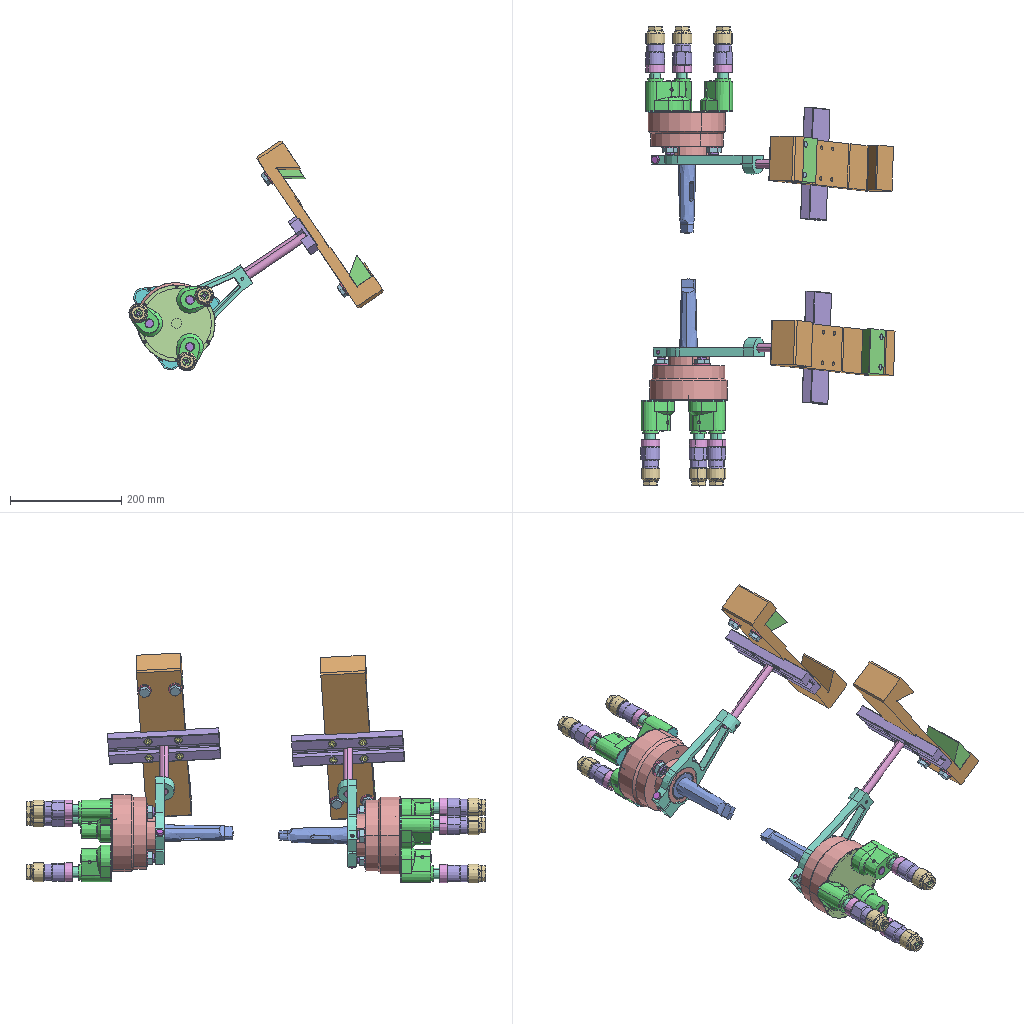Assembly | SolidWorks | 34 different items | 143 placed | box 457 x 827 x 414 mm
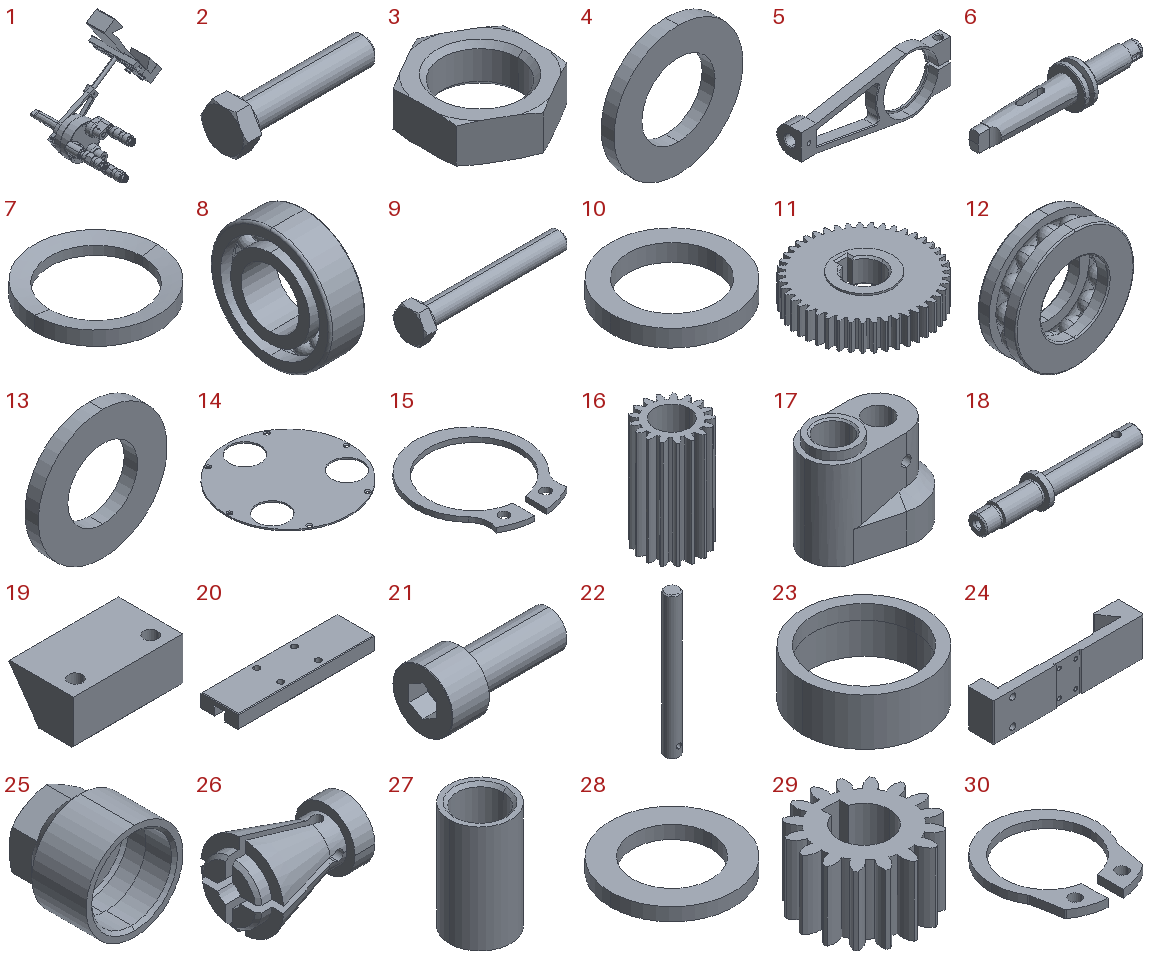Parts list (item | name | quantity | parent item | size | volume | features):
1 | (subassembly) | x2 | - | 456.998 x 372.31 x 409.469 mm | 2395331 mm3 | features ReferencePattern 32, CompositeCurve 27, LocalCirPattern 3
2 | - | x4 | in 1 | 62.5 x 20.785 x 18 mm | 8272 mm3 | features RevCut 4, Chamfer 1, Extrusion 1, Fillet 1, LPattern 1, Revolution 1
3 | - | x6 | in 1 | 23.219 x 26.75 x 8 mm | 2049 mm3 | features Cut 2, Chamfer 1, Extrusion 1
4 | - | x6 | in 1 | 30 x 3 x 30 mm | 1440 mm3 | features Revolution 1
5 | - | x2 | in 1 | 210 x 34 x 82 mm | 81908 mm3 | features ICE 6, Chamfer 3, Fillet 2, HoleWzd 2, CutThin 1, ExtruRefSurface 1, Extrusion 1
6 | - | x2 | in 1 | 216 x 51 x 51 mm | 132474 mm3 | features ICE 5, Chamfer 1, MirrorPattern 1, Revolution 1, SweepCut 1
7 | - | x2 | in 1 | 52 x 52 x 6 mm | 4561 mm3 | features Extrusion 1, ICE 1, MirrorPattern 1
8 | - | x4 | in 1 | 15 x 52 x 52 mm | 16133 mm3 | features Revolution 3, Fillet 2, CirPattern 1
9 | - | x2 | in 1 | 65.3 x 15.011 x 13 mm | 3770 mm3 | features RevCut 4, Chamfer 1, Extrusion 1, Fillet 1, LPattern 1, Revolution 1
10 | - | x2 | in 1 | 36 x 36 x 5 mm | 2536 mm3 | features Extrusion 1
11 | - | x2 | in 1 | 70.282 x 70.32 x 16 mm | 46691 mm3 | features ICE 4, Chamfer 1, CirPattern 1, Extrusion 1
12 | - | x6 | in 1 | 28 x 9 x 28 mm | 2845 mm3 | features Revolution 3, CirPattern 1, Fillet 1
13 | - | x4 | in 1 | 24 x 2.5 x 24 mm | 799.143 mm3 | features Revolution 1
14 | - | x2 | in 1 | 139 x 139 x 1.5 mm | 18307 mm3 | features ICE 3, CirPattern 2, Extrusion 1
15 | - | x6 | in 1 | 22.5 x 25.566 x 1 mm | 158.597 mm3 | features Extrusion 1
16 | - | x6 | in 1 | 28.328 x 28.443 x 49.5 mm | 14667 mm3 | features CirPattern 1, Extrusion 1, ICE 1
17 | - | x6 | in 1 | 68 x 48 x 58 mm | 60377 mm3 | features ICE 7, Chamfer 2, Extrusion 1, HoleWzd 1
18 | - | x6 | in 1 | 133 x 25 x 25 mm | 28520 mm3 | features ICE 3, Chamfer 2, RevCut 1, Revolution 1
19 | - | x2 | in 1 | 80 x 46.833 x 32 mm | 87358 mm3 | features Chamfer 1, Extrusion 1, HoleWzd 1, MirrorPattern 1
20 | - | x2 | in 1 | 200 x 55 x 20 mm | 170246 mm3 | features MirrorPattern 2, Chamfer 1, Extrusion 1, HoleWzd 1
21 | - | x8 | in 1 | 28 x 13 x 13 mm | 1937 mm3 | features BlendCut 1, Cut 1, Fillet 1, LPattern 1, RevCut 1, Revolution 1
22 | - | x2 | in 1 | 15 x 15 x 150 mm | 26172 mm3 | features Chamfer 1, ExtruRefSurface 1, Extrusion 1, HoleWzd 1
23 | - | x6 | in 1 | 34 x 34 x 13 mm | 3395 mm3 | features Extrusion 1, ICE 1
24 | - | x2 | in 1 | 320 x 55 x 80 mm | 674156 mm3 | features ICE 3, MirrorPattern 2, Chamfer 1, Extrusion 1, HoleWzd 1
25 | - | x6 | in 1 | 34 x 32 x 34 mm | 9791 mm3 | features ICE 6, Chamfer 2, Extrusion 1, HoleWzd 1
26 | - | x6 | in 1 | 35 x 24.92 x 24.92 mm | 6477 mm3 | features ICE 5, Chamfer 1, Revolution 1
27 | - | x6 | in 1 | 20 x 20 x 35 mm | 4761 mm3 | features Chamfer 1, Extrusion 1
28 | - | x6 | in 1 | 23.5 x 23.5 x 2.5 mm | 642.554 mm3 | features Extrusion 1
29 | - | x6 | in 1 | 26.937 x 26.937 x 16 mm | 5099 mm3 | features ICE 2, CirPattern 1, Extrusion 1
30 | - | x6 | in 1 | 13.6 x 15.973 x 1 mm | 68.14 mm3 | features Extrusion 1
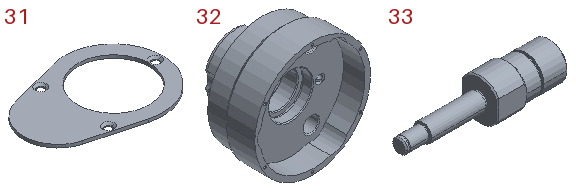31 | - | x6 | in 1 | 68 x 48 x 1.5 mm | 2249 mm3 | features ICE 5, Extrusion 1
32 | - | x2 | in 1 | 139 x 94 x 139 mm | 531526 mm3 | features Chamfer 3, ICE 3, CirPattern 2, RevCut 2, SweepCut 2, HoleWzd 1, Revolution 1
33 | - | x6 | in 1 | 124 x 30 x 34 mm | 43283 mm3 | features Chamfer 2, ICE 2, RevCut 1, Revolution 1
34 | Base Plate | x1 | - | - | - | -
Mates (type | each side: item.copy, entity, surface, feature):
Concentric | 6.1 edge | 7.1 edge
Coincident | 6.1 face cone Revolve1 | 7.1 edge
Concentric | 32.1 edge | 6.1 edge
Coincident | 32.1 face plane Revolve1 | 6.1 face plane Revolve1
Concentric | 32.1 edge | 5.1 edge
Coincident | 32.1 face plane Revolve1 | 5.1 face plane Cut-Extrude3
Concentric | 22.1 edge | 5.1 edge
Coincident | 22.1 face plane Boss-Extrude1 | 5.1 face plane Boss-Extrude2
Concentric | 22.1 face cylinder Ø5.0mm Blind Hole1 | 5.1 face cylinder Ø5.0mm Blind Hole1
Coincident | 22.1 face plane Boss-Extrude1 | 20.1 face plane Boss-Extrude1
Width | 20.1 face plane Boss-Extrude1 | 20.1 face plane Boss-Extrude1 | 22.1 face cylinder Boss-Extrude1 | 2 times
Coincident | 24.1 face plane Cut-Extrude2 | 20.1 face plane Boss-Extrude1
Concentric | 24.1 edge | 20.1 edge | 2 times
Coincident | 24.1 face plane Cut-Extrude1 | 19.1 face plane Boss-Extrude1
Concentric | 24.1 face cylinder Cut-Extrude3 | 19.1 edge | 2 times
Concentric | 24.1 face cylinder Cut-Extrude3 | 2.1 face cylinder Boss-Revolve1
Coincident | 19.1 face plane Boss-Extrude1 | 2.1 face plane Boss-Revolve1
Coincident | 24.1 face plane Boss-Extrude1 | 13.1 face plane Base-Revolve
Concentric | 13.1 face cylinder Base-Revolve | 2.1 face cylinder Boss-Revolve1
Concentric | 2.2 face cylinder Boss-Revolve1 | 13.2 face cylinder Base-Revolve
Coincident | 2.2 face plane Base-Extrude | 13.2 face plane Base-Revolve
Concentric | 24.1 face cylinder Cut-Extrude3 | 2.2 face cylinder Boss-Revolve1
Coincident | 19.1 face plane Boss-Extrude1 | 2.2 face plane Boss-Revolve1
Concentric | 24.1 face cylinder Mirror2 | 21.1 face cylinder Base-Revolve
Coincident | 20.1 face plane Mirror2 | 21.1 face plane Base-Revolve
Concentric | 20.1 face cylinder Mirror2 | 21.2 face cylinder Base-Revolve
Concentric | 20.1 face cylinder Hole5 | 21.3 face cylinder Base-Revolve
Concentric | 20.1 face cylinder Mirror1 | 21.4 face cylinder Base-Revolve
Coincident | 20.1 face plane Mirror1 | 21.4 face plane Base-Revolve
Coincident | 20.1 face plane Hole5 | 21.3 face plane Base-Revolve
Coincident | 20.1 face plane Mirror2 | 21.2 face plane Base-Revolve
Concentric | 5.1 face cylinder Cut-Extrude4 | 9.1 face cylinder Boss-Revolve1
Coincident | 5.1 face plane Boss-Extrude1 | 9.1 face plane Base-Extrude
Concentric | 6.1 face cylinder Revolve1 | 8.1 face cylinder Base-Revolve
Coincident | 32.1 face plane Cut-Revolve1 | 8.1 face plane Base-Revolve
Concentric | 32.1 face cylinder Cut-Revolve1 | 11.1 face cylinder Cut-Extrude2
Concentric | 6.1 face cylinder Revolve1 | 8.2 face cylinder Boss-Revolve2
Concentric | 6.1 face cylinder Revolve1 | 10.1 face cylinder Boss-Extrude1
Coincident | 32.1 face plane Cut-Revolve1 | 8.2 face plane Base-Revolve
Coincident | 8.2 face plane Boss-Revolve2 | 10.1 face plane Boss-Extrude1
Coincident | 11.1 face plane Cut-Extrude2 | 10.1 face plane Boss-Extrude1
Concentric | 32.1 face cylinder Revolve1 | 14.1 face cylinder Boss-Extrude1
Concentric | 32.1 edge | 14.1 edge
Concentric | 6.1 edge | 15.1 edge
Coincident | 6.1 face plane Revolve1 | 15.1 face plane Base-Extrude
Coincident | 32.1 face plane Revolve1 | 14.1 face plane Boss-Extrude1
Concentric | 31.1 edge | 17.1 edge | 2 times
Coincident | 31.1 face plane Boss-Extrude1 | 17.1 face plane Boss-Extrude1
Concentric | 14.1 face cylinder Cut-Extrude1 | 31.1 face cylinder Cut-Extrude1
Coincident | 14.1 face plane Boss-Extrude1 | 31.1 face plane Boss-Extrude1
Concentric | 18.1 face cylinder Revolve1 | 17.1 face cylinder Cut-Extrude3
Concentric | 18.1 face cylinder Cut-Extrude1 | 17.1 face cylinder Cut-Extrude5
Concentric | 17.1 edge | 29.1 edge
Concentric | 17.1 face cylinder Cut-Extrude1 | 30.1 edge
Concentric | 25.1 face cylinder M30x2.0 Tapped Hole1 | 17.1 face cylinder Cut-Extrude1
Concentric | 17.1 face cylinder Cut-Extrude1 | 28.1 face cylinder Boss-Extrude1
Concentric | 17.1 face cylinder Cut-Extrude1 | 27.1 face cylinder Boss-Extrude1
Concentric | 17.1 face cylinder Cut-Extrude1 | 23.1 face cylinder Cut-Extrude1
Concentric | 17.1 face cylinder Cut-Extrude1 | 33.1 face cylinder Revolve1
Coincident | 30.1 face plane Base-Extrude | 33.1 face plane Revolve1
Concentric | 12.1 face cylinder Boss-Revolve3 | 33.1 face cylinder Revolve1
Coincident | 12.1 face plane Base-Revolve | 33.1 face plane Revolve1
Coincident | 29.1 face plane Boss-Extrude1 | 33.1 face plane Revolve1
Coincident | 29.1 face plane Boss-Extrude1 | 28.1 face plane Boss-Extrude1
Coincident | 28.1 face plane Boss-Extrude1 | 27.1 face plane Boss-Extrude1
Coincident | 23.1 face plane Boss-Extrude1 | 33.1 face plane Revolve1
Concentric | 33.1 face cone Cut-Revolve1 | 26.1 face cylinder Revolve1
Coincident | 33.1 edge | 26.1 face plane Revolve1
Coincident | 25.1 face plane Boss-Extrude2 | 33.1 face plane Revolve1
Coincident | 4.1 face plane Base-Revolve | 3.1 face plane Base-Extrude
Concentric | 4.1 face cylinder Base-Revolve | 3.1 face cylinder Base-Extrude
Concentric | 18.2 face cylinder Revolve1 | 3.1 face cylinder Base-Extrude
Coincident | 32.1 face plane Revolve1 | 4.1 face plane Base-Revolve
Concentric | 18.2 face cylinder Revolve1 | 16.1 face cylinder Boss-Extrude1
Coincident | 17.2 face plane Cut-Extrude2 | 16.1 face plane Boss-Extrude1